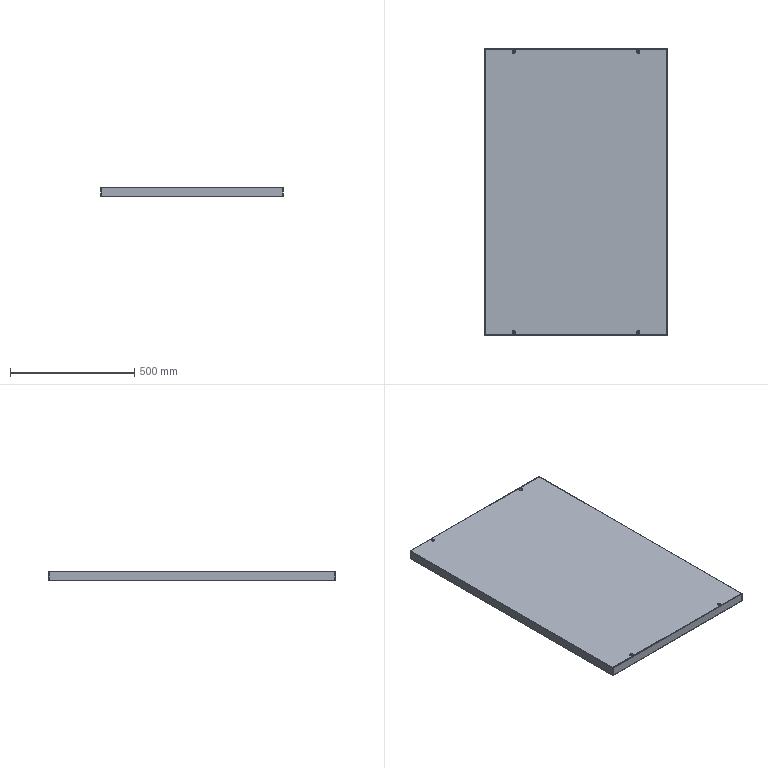Part | STEP file | SX-021-01 | 1 solid | 86 faces | box 736.001 x 1156 x 39 mm | volume 2140598 mm3 | plane 42 | cylinder 32 | spline 12 | commonest cylinder face diameters 0.4 x8 4.4 x8 8 x8 14 x8